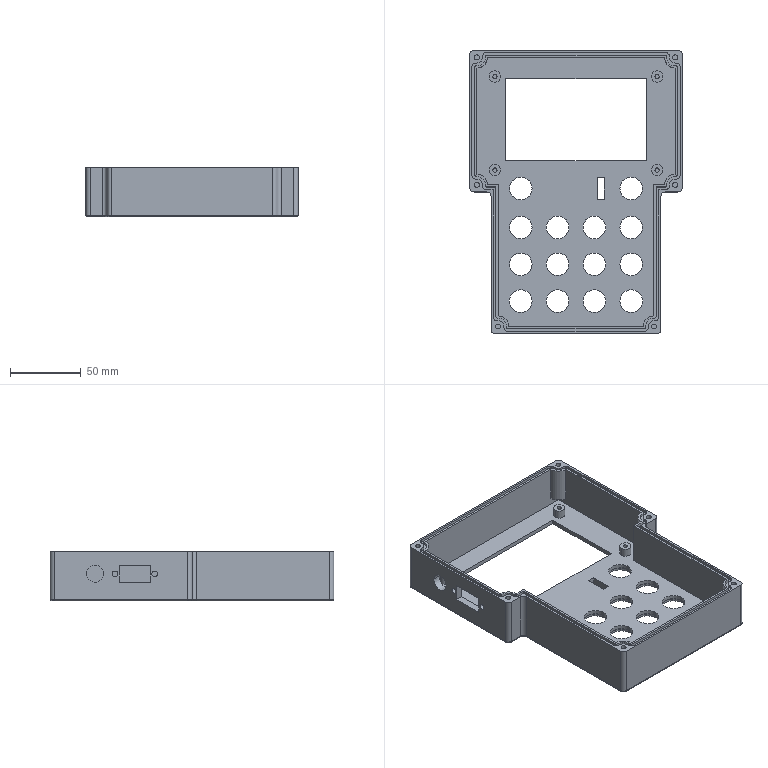Part | SolidWorks | features ICE 9, Fillet 2, Chamfer 1, Extrusion 1 | 1 solid | 257 faces | box 150 x 200 x 35 mm | volume 192562 mm3 | cylinder 160 | plane 89 | torus 8 | commonest cylinder face diameters 16 x28 17 x28 2 x23 6 x23 8 x17 3.5 x12